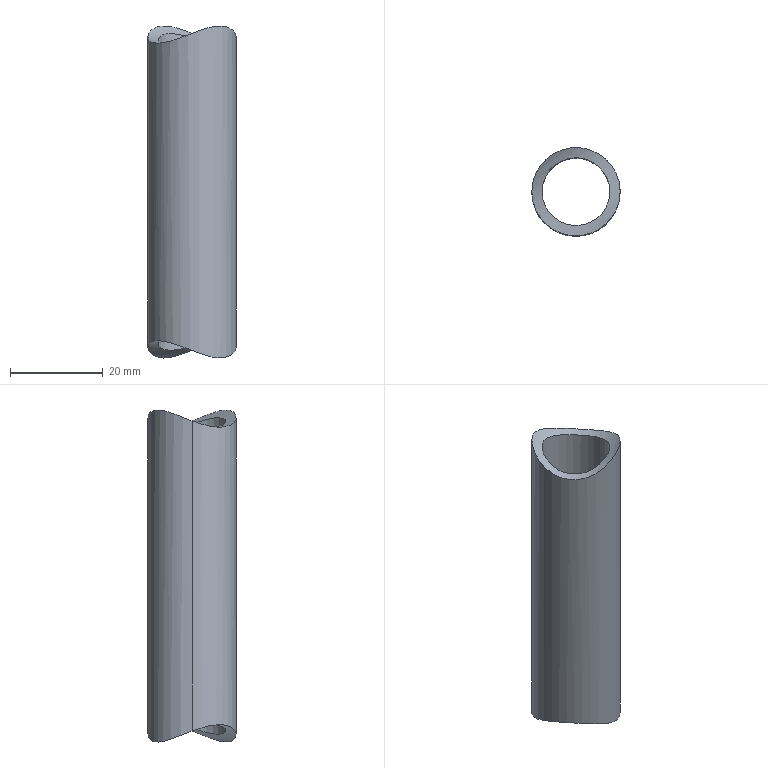Part | STEP file | PRT0001_68_6 | 1 solid | 6 faces | box 19.001 x 19.001 x 71.436 mm | volume 7755 mm3 | cylinder 6 | commonest cylinder face diameters 14.601 x2 19.001 x2 28 x2